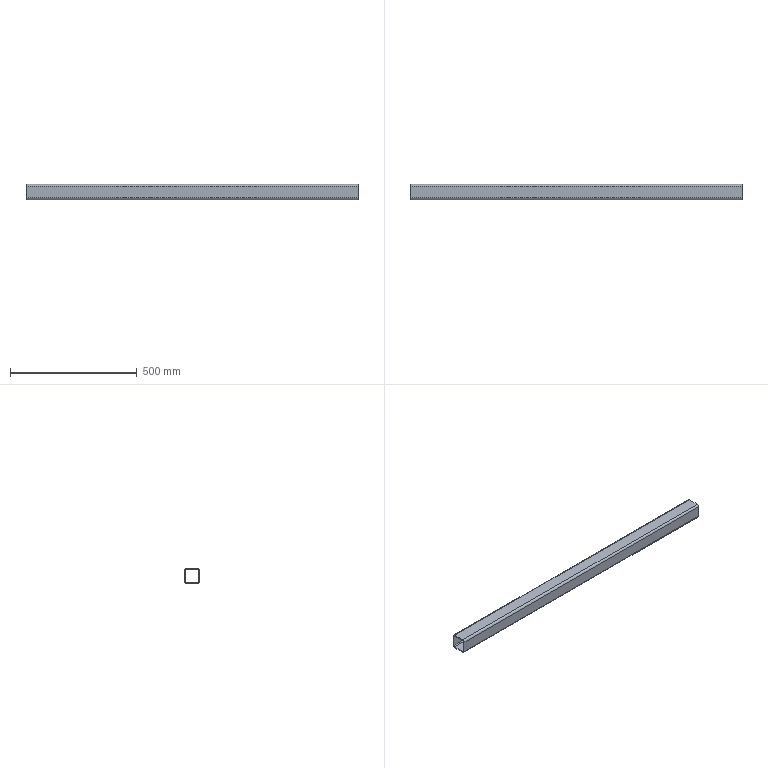Part | SolidWorks | features BaseBody 1 | 1 solid | 18 faces | box 1310 x 60 x 60 mm | volume 1119783 mm3 | plane 10 | cylinder 8 | commonest cylinder face diameters 8 x4 16 x4
STEP:
#1=CARTESIAN_POINT('',(670.,2436.,552.));
#2=VERTEX_POINT('',#1);
#3=CARTESIAN_POINT('',(670.,2436.,508.));
#4=VERTEX_POINT('',#3);
#5=CARTESIAN_POINT('',(670.,2436.,508.));
#6=DIRECTION('',(0.,0.,-1.));
#7=VECTOR('',#6,1000.);
#8=LINE('',#5,#7);
#9=EDGE_CURVE('',#2,#4,#8,.T.);
#10=ORIENTED_EDGE('',*,*,#9,.T.);
#11=CARTESIAN_POINT('',(-640.,2436.,508.));
#12=VERTEX_POINT('',#11);
#13=CARTESIAN_POINT('',(670.,2436.,508.));
#14=DIRECTION('',(-1.,0.,0.));
#15=VECTOR('',#14,1000.);
#16=LINE('',#13,#15);
#17=EDGE_CURVE('',#4,#12,#16,.T.);
#18=ORIENTED_EDGE('',*,*,#17,.T.);
#19=CARTESIAN_POINT('',(-640.,2436.,552.));
#20=VERTEX_POINT('',#19);
#21=CARTESIAN_POINT('',(-640.,2436.,508.));
#22=DIRECTION('',(0.,0.,1.));
#23=VECTOR('',#22,1000.);
#24=LINE('',#21,#23);
#25=EDGE_CURVE('',#12,#20,#24,.T.);
#26=ORIENTED_EDGE('',*,*,#25,.T.);
#27=CARTESIAN_POINT('',(670.,2436.,552.));
#28=DIRECTION('',(1.,0.,0.));
#29=VECTOR('',#28,1000.);
#30=LINE('',#27,#29);
#31=EDGE_CURVE('',#20,#2,#30,.T.);
#32=ORIENTED_EDGE('',*,*,#31,.T.);
#33=EDGE_LOOP('',(#10,#18,#26,#32));
#34=FACE_OUTER_BOUND('',#33,.T.);
#35=CARTESIAN_POINT('',(670.,2436.,508.));
#36=DIRECTION('',(0.,1.,0.));
#37=DIRECTION('',(0.,0.,1.));
#38=AXIS2_PLACEMENT_3D('',#35,#36,#37);
#39=PLANE('',#38);
#40=ADVANCED_FACE('',(#34),#39,.T.);
#41=ORIENTED_EDGE('',*,*,#17,.F.);
#42=CARTESIAN_POINT('',(670.,2440.,504.));
#43=VERTEX_POINT('',#42);
#44=CARTESIAN_POINT('',(670.,2440.,508.));
#45=DIRECTION('',(-1.,0.,0.));
#46=DIRECTION('',(0.,0.,1.));
#47=AXIS2_PLACEMENT_3D('',#44,#45,#46);
#48=CIRCLE('',#47,4.);
#49=EDGE_CURVE('',#43,#4,#48,.T.);
#50=ORIENTED_EDGE('',*,*,#49,.F.);
#51=CARTESIAN_POINT('',(-640.,2440.,504.));
#52=VERTEX_POINT('',#51);
#53=CARTESIAN_POINT('',(670.,2440.,504.));
#54=DIRECTION('',(1.,0.,0.));
#55=VECTOR('',#54,1000.);
#56=LINE('',#53,#55);
#57=EDGE_CURVE('',#52,#43,#56,.T.);
#58=ORIENTED_EDGE('',*,*,#57,.F.);
#59=CARTESIAN_POINT('',(-640.,2440.,508.));
#60=DIRECTION('',(1.,0.,0.));
#61=DIRECTION('',(0.,0.,1.));
#62=AXIS2_PLACEMENT_3D('',#59,#60,#61);
#63=CIRCLE('',#62,4.);
#64=EDGE_CURVE('',#12,#52,#63,.T.);
#65=ORIENTED_EDGE('',*,*,#64,.F.);
#66=EDGE_LOOP('',(#41,#50,#58,#65));
#67=FACE_OUTER_BOUND('',#66,.T.);
#68=CARTESIAN_POINT('',(670.,2440.,508.));
#69=DIRECTION('',(-1.,0.,0.));
#70=DIRECTION('',(0.,0.,1.));
#71=AXIS2_PLACEMENT_3D('',#68,#69,#70);
#72=CYLINDRICAL_SURFACE('',#71,4.);
#73=ADVANCED_FACE('',(#67),#72,.F.);
#74=ORIENTED_EDGE('',*,*,#9,.F.);
#75=CARTESIAN_POINT('',(670.,2440.,556.));
#76=VERTEX_POINT('',#75);
#77=CARTESIAN_POINT('',(670.,2440.,552.));
#78=DIRECTION('',(-1.,0.,0.));
#79=DIRECTION('',(0.,0.,1.));
#80=AXIS2_PLACEMENT_3D('',#77,#78,#79);
#81=CIRCLE('',#80,4.);
#82=EDGE_CURVE('',#2,#76,#81,.T.);
#83=ORIENTED_EDGE('',*,*,#82,.T.);
#84=CARTESIAN_POINT('',(670.,2484.,556.));
#85=VERTEX_POINT('',#84);
#86=CARTESIAN_POINT('',(670.,2484.,556.));
#87=DIRECTION('',(0.,1.,0.));
#88=VECTOR('',#87,1000.);
#89=LINE('',#86,#88);
#90=EDGE_CURVE('',#76,#85,#89,.T.);
#91=ORIENTED_EDGE('',*,*,#90,.T.);
#92=CARTESIAN_POINT('',(670.,2488.,552.));
#93=VERTEX_POINT('',#92);
#94=CARTESIAN_POINT('',(670.,2484.,552.));
#95=DIRECTION('',(-1.,0.,0.));
#96=DIRECTION('',(0.,0.,1.));
#97=AXIS2_PLACEMENT_3D('',#94,#95,#96);
#98=CIRCLE('',#97,4.);
#99=EDGE_CURVE('',#85,#93,#98,.T.);
#100=ORIENTED_EDGE('',*,*,#99,.T.);
#101=CARTESIAN_POINT('',(670.,2488.,508.));
#102=VERTEX_POINT('',#101);
#103=CARTESIAN_POINT('',(670.,2488.,552.));
#104=DIRECTION('',(0.,0.,-1.));
#105=VECTOR('',#104,1000.);
#106=LINE('',#103,#105);
#107=EDGE_CURVE('',#93,#102,#106,.T.);
#108=ORIENTED_EDGE('',*,*,#107,.T.);
#109=CARTESIAN_POINT('',(670.,2484.,504.));
#110=VERTEX_POINT('',#109);
#111=CARTESIAN_POINT('',(670.,2484.,508.));
#112=DIRECTION('',(-1.,0.,0.));
#113=DIRECTION('',(0.,0.,1.));
#114=AXIS2_PLACEMENT_3D('',#111,#112,#113);
#115=CIRCLE('',#114,4.);
#116=EDGE_CURVE('',#102,#110,#115,.T.);
#117=ORIENTED_EDGE('',*,*,#116,.T.);
#118=CARTESIAN_POINT('',(670.,2484.,504.));
#119=DIRECTION('',(0.,-1.,0.));
#120=VECTOR('',#119,1000.);
#121=LINE('',#118,#120);
#122=EDGE_CURVE('',#110,#43,#121,.T.);
#123=ORIENTED_EDGE('',*,*,#122,.T.);
#124=ORIENTED_EDGE('',*,*,#49,.T.);
#125=EDGE_LOOP('',(#74,#83,#91,#100,#108,#117,#123,#124));
#126=FACE_BOUND('',#125,.T.);
#127=CARTESIAN_POINT('',(670.,2492.,508.));
#128=VERTEX_POINT('',#127);
#129=CARTESIAN_POINT('',(670.,2492.,552.));
#130=VERTEX_POINT('',#129);
#131=CARTESIAN_POINT('',(670.,2492.,552.));
#132=DIRECTION('',(0.,0.,1.));
#133=VECTOR('',#132,1000.);
#134=LINE('',#131,#133);
#135=EDGE_CURVE('',#128,#130,#134,.T.);
#136=ORIENTED_EDGE('',*,*,#135,.T.);
#137=CARTESIAN_POINT('',(670.,2484.,560.));
#138=VERTEX_POINT('',#137);
#139=CARTESIAN_POINT('',(670.,2484.,552.));
#140=DIRECTION('',(1.,0.,0.));
#141=DIRECTION('',(0.,0.,1.));
#142=AXIS2_PLACEMENT_3D('',#139,#140,#141);
#143=CIRCLE('',#142,8.);
#144=EDGE_CURVE('',#130,#138,#143,.T.);
#145=ORIENTED_EDGE('',*,*,#144,.T.);
#146=CARTESIAN_POINT('',(670.,2440.,560.));
#147=VERTEX_POINT('',#146);
#148=CARTESIAN_POINT('',(670.,2484.,560.));
#149=DIRECTION('',(0.,-1.,0.));
#150=VECTOR('',#149,1000.);
#151=LINE('',#148,#150);
#152=EDGE_CURVE('',#138,#147,#151,.T.);
#153=ORIENTED_EDGE('',*,*,#152,.T.);
#154=CARTESIAN_POINT('',(670.,2432.,552.));
#155=VERTEX_POINT('',#154);
#156=CARTESIAN_POINT('',(670.,2440.,552.));
#157=DIRECTION('',(1.,0.,0.));
#158=DIRECTION('',(0.,0.,1.));
#159=AXIS2_PLACEMENT_3D('',#156,#157,#158);
#160=CIRCLE('',#159,8.);
#161=EDGE_CURVE('',#147,#155,#160,.T.);
#162=ORIENTED_EDGE('',*,*,#161,.T.);
#163=CARTESIAN_POINT('',(670.,2432.,508.));
#164=VERTEX_POINT('',#163);
#165=CARTESIAN_POINT('',(670.,2432.,552.));
#166=DIRECTION('',(0.,0.,-1.));
#167=VECTOR('',#166,1000.);
#168=LINE('',#165,#167);
#169=EDGE_CURVE('',#155,#164,#168,.T.);
#170=ORIENTED_EDGE('',*,*,#169,.T.);
#171=CARTESIAN_POINT('',(670.,2440.,500.));
#172=VERTEX_POINT('',#171);
#173=CARTESIAN_POINT('',(670.,2440.,508.));
#174=DIRECTION('',(1.,0.,0.));
#175=DIRECTION('',(0.,0.,1.));
#176=AXIS2_PLACEMENT_3D('',#173,#174,#175);
#177=CIRCLE('',#176,8.);
#178=EDGE_CURVE('',#164,#172,#177,.T.);
#179=ORIENTED_EDGE('',*,*,#178,.T.);
#180=CARTESIAN_POINT('',(670.,2484.,500.));
#181=VERTEX_POINT('',#180);
#182=CARTESIAN_POINT('',(670.,2484.,500.));
#183=DIRECTION('',(0.,1.,0.));
#184=VECTOR('',#183,1000.);
#185=LINE('',#182,#184);
#186=EDGE_CURVE('',#172,#181,#185,.T.);
#187=ORIENTED_EDGE('',*,*,#186,.T.);
#188=CARTESIAN_POINT('',(670.,2484.,508.));
#189=DIRECTION('',(1.,0.,0.));
#190=DIRECTION('',(0.,0.,1.));
#191=AXIS2_PLACEMENT_3D('',#188,#189,#190);
#192=CIRCLE('',#191,8.);
#193=EDGE_CURVE('',#181,#128,#192,.T.);
#194=ORIENTED_EDGE('',*,*,#193,.T.);
#195=EDGE_LOOP('',(#136,#145,#153,#162,#170,#179,#187,#194));
#196=FACE_OUTER_BOUND('',#195,.T.);
#197=CARTESIAN_POINT('',(670.,2484.,552.));
#198=DIRECTION('',(1.,0.,0.));
#199=DIRECTION('',(0.,0.,-1.));
#200=AXIS2_PLACEMENT_3D('',#197,#198,#199);
#201=PLANE('',#200);
#202=ADVANCED_FACE('',(#126,#196),#201,.T.);
#203=CARTESIAN_POINT('',(-640.,2440.,556.));
#204=VERTEX_POINT('',#203);
#205=CARTESIAN_POINT('',(670.,2440.,556.));
#206=DIRECTION('',(-1.,0.,0.));
#207=VECTOR('',#206,1000.);
#208=LINE('',#205,#207);
#209=EDGE_CURVE('',#76,#204,#208,.T.);
#210=ORIENTED_EDGE('',*,*,#209,.F.);
#211=ORIENTED_EDGE('',*,*,#82,.F.);
#212=ORIENTED_EDGE('',*,*,#31,.F.);
#213=CARTESIAN_POINT('',(-640.,2440.,552.));
#214=DIRECTION('',(1.,0.,0.));
#215=DIRECTION('',(0.,0.,1.));
#216=AXIS2_PLACEMENT_3D('',#213,#214,#215);
#217=CIRCLE('',#216,4.);
#218=EDGE_CURVE('',#204,#20,#217,.T.);
#219=ORIENTED_EDGE('',*,*,#218,.F.);
#220=EDGE_LOOP('',(#210,#211,#212,#219));
#221=FACE_OUTER_BOUND('',#220,.T.);
#222=CARTESIAN_POINT('',(670.,2440.,552.));
#223=DIRECTION('',(-1.,0.,0.));
#224=DIRECTION('',(0.,0.,1.));
#225=AXIS2_PLACEMENT_3D('',#222,#223,#224);
#226=CYLINDRICAL_SURFACE('',#225,4.);
#227=ADVANCED_FACE('',(#221),#226,.F.);
#228=ORIENTED_EDGE('',*,*,#218,.T.);
#229=ORIENTED_EDGE('',*,*,#25,.F.);
#230=ORIENTED_EDGE('',*,*,#64,.T.);
#231=CARTESIAN_POINT('',(-640.,2484.,504.));
#232=VERTEX_POINT('',#231);
#233=CARTESIAN_POINT('',(-640.,2440.,504.));
#234=DIRECTION('',(0.,1.,0.));
#235=VECTOR('',#234,1000.);
#236=LINE('',#233,#235);
#237=EDGE_CURVE('',#52,#232,#236,.T.);
#238=ORIENTED_EDGE('',*,*,#237,.T.);
#239=CARTESIAN_POINT('',(-640.,2488.,508.));
#240=VERTEX_POINT('',#239);
#241=CARTESIAN_POINT('',(-640.,2484.,508.));
#242=DIRECTION('',(1.,0.,0.));
#243=DIRECTION('',(0.,0.,1.));
#244=AXIS2_PLACEMENT_3D('',#241,#242,#243);
#245=CIRCLE('',#244,4.);
#246=EDGE_CURVE('',#232,#240,#245,.T.);
#247=ORIENTED_EDGE('',*,*,#246,.T.);
#248=CARTESIAN_POINT('',(-640.,2488.,552.));
#249=VERTEX_POINT('',#248);
#250=CARTESIAN_POINT('',(-640.,2488.,-1270.));
#251=DIRECTION('',(0.,0.,1.));
#252=VECTOR('',#251,1000.);
#253=LINE('',#250,#252);
#254=EDGE_CURVE('',#240,#249,#253,.T.);
#255=ORIENTED_EDGE('',*,*,#254,.T.);
#256=CARTESIAN_POINT('',(-640.,2484.,556.));
#257=VERTEX_POINT('',#256);
#258=CARTESIAN_POINT('',(-640.,2484.,552.));
#259=DIRECTION('',(1.,0.,0.));
#260=DIRECTION('',(0.,0.,1.));
#261=AXIS2_PLACEMENT_3D('',#258,#259,#260);
#262=CIRCLE('',#261,4.);
#263=EDGE_CURVE('',#249,#257,#262,.T.);
#264=ORIENTED_EDGE('',*,*,#263,.T.);
#265=CARTESIAN_POINT('',(-640.,2440.,556.));
#266=DIRECTION('',(0.,-1.,0.));
#267=VECTOR('',#266,1000.);
#268=LINE('',#265,#267);
#269=EDGE_CURVE('',#257,#204,#268,.T.);
#270=ORIENTED_EDGE('',*,*,#269,.T.);
#271=EDGE_LOOP('',(#228,#229,#230,#238,#247,#255,#264,#270));
#272=FACE_BOUND('',#271,.T.);
#273=CARTESIAN_POINT('',(-640.,2440.,560.));
#274=VERTEX_POINT('',#273);
#275=CARTESIAN_POINT('',(-640.,2484.,560.));
#276=VERTEX_POINT('',#275);
#277=CARTESIAN_POINT('',(-640.,2440.,560.));
#278=DIRECTION('',(0.,1.,0.));
#279=VECTOR('',#278,1000.);
#280=LINE('',#277,#279);
#281=EDGE_CURVE('',#274,#276,#280,.T.);
#282=ORIENTED_EDGE('',*,*,#281,.T.);
#283=CARTESIAN_POINT('',(-640.,2492.,552.));
#284=VERTEX_POINT('',#283);
#285=CARTESIAN_POINT('',(-640.,2484.,552.));
#286=DIRECTION('',(-1.,0.,0.));
#287=DIRECTION('',(0.,0.,1.));
#288=AXIS2_PLACEMENT_3D('',#285,#286,#287);
#289=CIRCLE('',#288,8.);
#290=EDGE_CURVE('',#276,#284,#289,.T.);
#291=ORIENTED_EDGE('',*,*,#290,.T.);
#292=CARTESIAN_POINT('',(-640.,2492.,508.));
#293=VERTEX_POINT('',#292);
#294=CARTESIAN_POINT('',(-640.,2492.,-1270.));
#295=DIRECTION('',(0.,0.,-1.));
#296=VECTOR('',#295,1000.);
#297=LINE('',#294,#296);
#298=EDGE_CURVE('',#284,#293,#297,.T.);
#299=ORIENTED_EDGE('',*,*,#298,.T.);
#300=CARTESIAN_POINT('',(-640.,2484.,500.));
#301=VERTEX_POINT('',#300);
#302=CARTESIAN_POINT('',(-640.,2484.,508.));
#303=DIRECTION('',(-1.,0.,0.));
#304=DIRECTION('',(0.,0.,1.));
#305=AXIS2_PLACEMENT_3D('',#302,#303,#304);
#306=CIRCLE('',#305,8.);
#307=EDGE_CURVE('',#293,#301,#306,.T.);
#308=ORIENTED_EDGE('',*,*,#307,.T.);
#309=CARTESIAN_POINT('',(-640.,2440.,500.));
#310=VERTEX_POINT('',#309);
#311=CARTESIAN_POINT('',(-640.,2440.,500.));
#312=DIRECTION('',(0.,-1.,0.));
#313=VECTOR('',#312,1000.);
#314=LINE('',#311,#313);
#315=EDGE_CURVE('',#301,#310,#314,.T.);
#316=ORIENTED_EDGE('',*,*,#315,.T.);
#317=CARTESIAN_POINT('',(-640.,2432.,508.));
#318=VERTEX_POINT('',#317);
#319=CARTESIAN_POINT('',(-640.,2440.,508.));
#320=DIRECTION('',(-1.,0.,0.));
#321=DIRECTION('',(0.,0.,1.));
#322=AXIS2_PLACEMENT_3D('',#319,#320,#321);
#323=CIRCLE('',#322,8.);
#324=EDGE_CURVE('',#310,#318,#323,.T.);
#325=ORIENTED_EDGE('',*,*,#324,.T.);
#326=CARTESIAN_POINT('',(-640.,2432.,552.));
#327=VERTEX_POINT('',#326);
#328=CARTESIAN_POINT('',(-640.,2432.,-1270.));
#329=DIRECTION('',(0.,0.,1.));
#330=VECTOR('',#329,1000.);
#331=LINE('',#328,#330);
#332=EDGE_CURVE('',#318,#327,#331,.T.);
#333=ORIENTED_EDGE('',*,*,#332,.T.);
#334=CARTESIAN_POINT('',(-640.,2440.,552.));
#335=DIRECTION('',(-1.,0.,0.));
#336=DIRECTION('',(0.,0.,1.));
#337=AXIS2_PLACEMENT_3D('',#334,#335,#336);
#338=CIRCLE('',#337,8.);
#339=EDGE_CURVE('',#327,#274,#338,.T.);
#340=ORIENTED_EDGE('',*,*,#339,.T.);
#341=EDGE_LOOP('',(#282,#291,#299,#308,#316,#325,#333,#340));
#342=FACE_OUTER_BOUND('',#341,.T.);
#343=CARTESIAN_POINT('',(-640.,2440.,-1270.));
#344=DIRECTION('',(-1.,0.,0.));
#345=DIRECTION('',(0.,0.,1.));
#346=AXIS2_PLACEMENT_3D('',#343,#344,#345);
#347=PLANE('',#346);
#348=ADVANCED_FACE('',(#272,#342),#347,.T.);
#349=ORIENTED_EDGE('',*,*,#122,.F.);
#350=CARTESIAN_POINT('',(670.,2484.,504.));
#351=DIRECTION('',(-1.,0.,0.));
#352=VECTOR('',#351,1000.);
#353=LINE('',#350,#352);
#354=EDGE_CURVE('',#110,#232,#353,.T.);
#355=ORIENTED_EDGE('',*,*,#354,.T.);
#356=ORIENTED_EDGE('',*,*,#237,.F.);
#357=ORIENTED_EDGE('',*,*,#57,.T.);
#358=EDGE_LOOP('',(#349,#355,#356,#357));
#359=FACE_OUTER_BOUND('',#358,.T.);
#360=CARTESIAN_POINT('',(670.,2440.,504.));
#361=DIRECTION('',(0.,0.,1.));
#362=DIRECTION('',(1.,0.,0.));
#363=AXIS2_PLACEMENT_3D('',#360,#361,#362);
#364=PLANE('',#363);
#365=ADVANCED_FACE('',(#359),#364,.T.);
#366=ORIENTED_EDGE('',*,*,#354,.F.);
#367=ORIENTED_EDGE('',*,*,#116,.F.);
#368=CARTESIAN_POINT('',(670.,2488.,508.));
#369=DIRECTION('',(1.,0.,0.));
#370=VECTOR('',#369,1000.);
#371=LINE('',#368,#370);
#372=EDGE_CURVE('',#240,#102,#371,.T.);
#373=ORIENTED_EDGE('',*,*,#372,.F.);
#374=ORIENTED_EDGE('',*,*,#246,.F.);
#375=EDGE_LOOP('',(#366,#367,#373,#374));
#376=FACE_OUTER_BOUND('',#375,.T.);
#377=CARTESIAN_POINT('',(670.,2484.,508.));
#378=DIRECTION('',(-1.,0.,0.));
#379=DIRECTION('',(0.,0.,1.));
#380=AXIS2_PLACEMENT_3D('',#377,#378,#379);
#381=CYLINDRICAL_SURFACE('',#380,4.);
#382=ADVANCED_FACE('',(#376),#381,.F.);
#383=ORIENTED_EDGE('',*,*,#107,.F.);
#384=CARTESIAN_POINT('',(670.,2488.,552.));
#385=DIRECTION('',(-1.,0.,0.));
#386=VECTOR('',#385,1000.);
#387=LINE('',#384,#386);
#388=EDGE_CURVE('',#93,#249,#387,.T.);
#389=ORIENTED_EDGE('',*,*,#388,.T.);
#390=ORIENTED_EDGE('',*,*,#254,.F.);
#391=ORIENTED_EDGE('',*,*,#372,.T.);
#392=EDGE_LOOP('',(#383,#389,#390,#391));
#393=FACE_OUTER_BOUND('',#392,.T.);
#394=CARTESIAN_POINT('',(670.,2488.,552.));
#395=DIRECTION('',(0.,-1.,0.));
#396=DIRECTION('',(0.,0.,-1.));
#397=AXIS2_PLACEMENT_3D('',#394,#395,#396);
#398=PLANE('',#397);
#399=ADVANCED_FACE('',(#393),#398,.T.);
#400=ORIENTED_EDGE('',*,*,#388,.F.);
#401=ORIENTED_EDGE('',*,*,#99,.F.);
#402=CARTESIAN_POINT('',(670.,2484.,556.));
#403=DIRECTION('',(1.,0.,0.));
#404=VECTOR('',#403,1000.);
#405=LINE('',#402,#404);
#406=EDGE_CURVE('',#257,#85,#405,.T.);
#407=ORIENTED_EDGE('',*,*,#406,.F.);
#408=ORIENTED_EDGE('',*,*,#263,.F.);
#409=EDGE_LOOP('',(#400,#401,#407,#408));
#410=FACE_OUTER_BOUND('',#409,.T.);
#411=CARTESIAN_POINT('',(670.,2484.,552.));
#412=DIRECTION('',(-1.,0.,0.));
#413=DIRECTION('',(0.,0.,1.));
#414=AXIS2_PLACEMENT_3D('',#411,#412,#413);
#415=CYLINDRICAL_SURFACE('',#414,4.);
#416=ADVANCED_FACE('',(#410),#415,.F.);
#417=ORIENTED_EDGE('',*,*,#90,.F.);
#418=ORIENTED_EDGE('',*,*,#209,.T.);
#419=ORIENTED_EDGE('',*,*,#269,.F.);
#420=ORIENTED_EDGE('',*,*,#406,.T.);
#421=EDGE_LOOP('',(#417,#418,#419,#420));
#422=FACE_OUTER_BOUND('',#421,.T.);
#423=CARTESIAN_POINT('',(670.,2484.,556.));
#424=DIRECTION('',(0.,0.,-1.));
#425=DIRECTION('',(-1.,0.,0.));
#426=AXIS2_PLACEMENT_3D('',#423,#424,#425);
#427=PLANE('',#426);
#428=ADVANCED_FACE('',(#422),#427,.T.);
#429=CARTESIAN_POINT('',(670.,2492.,552.));
#430=DIRECTION('',(-1.,0.,0.));
#431=VECTOR('',#430,1000.);
#432=LINE('',#429,#431);
#433=EDGE_CURVE('',#130,#284,#432,.T.);
#434=ORIENTED_EDGE('',*,*,#433,.T.);
#435=ORIENTED_EDGE('',*,*,#290,.F.);
#436=CARTESIAN_POINT('',(670.,2484.,560.));
#437=DIRECTION('',(1.,0.,0.));
#438=VECTOR('',#437,1000.);
#439=LINE('',#436,#438);
#440=EDGE_CURVE('',#276,#138,#439,.T.);
#441=ORIENTED_EDGE('',*,*,#440,.T.);
#442=ORIENTED_EDGE('',*,*,#144,.F.);
#443=EDGE_LOOP('',(#434,#435,#441,#442));
#444=FACE_OUTER_BOUND('',#443,.T.);
#445=CARTESIAN_POINT('',(670.,2484.,552.));
#446=DIRECTION('',(-1.,0.,0.));
#447=DIRECTION('',(0.,0.,1.));
#448=AXIS2_PLACEMENT_3D('',#445,#446,#447);
#449=CYLINDRICAL_SURFACE('',#448,8.);
#450=ADVANCED_FACE('',(#444),#449,.T.);
#451=ORIENTED_EDGE('',*,*,#135,.F.);
#452=CARTESIAN_POINT('',(670.,2492.,508.));
#453=DIRECTION('',(1.,0.,0.));
#454=VECTOR('',#453,1000.);
#455=LINE('',#452,#454);
#456=EDGE_CURVE('',#293,#128,#455,.T.);
#457=ORIENTED_EDGE('',*,*,#456,.F.);
#458=ORIENTED_EDGE('',*,*,#298,.F.);
#459=ORIENTED_EDGE('',*,*,#433,.F.);
#460=EDGE_LOOP('',(#451,#457,#458,#459));
#461=FACE_OUTER_BOUND('',#460,.T.);
#462=CARTESIAN_POINT('',(670.,2492.,552.));
#463=DIRECTION('',(0.,-1.,0.));
#464=DIRECTION('',(0.,0.,-1.));
#465=AXIS2_PLACEMENT_3D('',#462,#463,#464);
#466=PLANE('',#465);
#467=ADVANCED_FACE('',(#461),#466,.F.);
#468=CARTESIAN_POINT('',(670.,2484.,500.));
#469=DIRECTION('',(-1.,0.,0.));
#470=VECTOR('',#469,1000.);
#471=LINE('',#468,#470);
#472=EDGE_CURVE('',#181,#301,#471,.T.);
#473=ORIENTED_EDGE('',*,*,#472,.T.);
#474=ORIENTED_EDGE('',*,*,#307,.F.);
#475=ORIENTED_EDGE('',*,*,#456,.T.);
#476=ORIENTED_EDGE('',*,*,#193,.F.);
#477=EDGE_LOOP('',(#473,#474,#475,#476));
#478=FACE_OUTER_BOUND('',#477,.T.);
#479=CARTESIAN_POINT('',(670.,2484.,508.));
#480=DIRECTION('',(-1.,0.,0.));
#481=DIRECTION('',(0.,0.,1.));
#482=AXIS2_PLACEMENT_3D('',#479,#480,#481);
#483=CYLINDRICAL_SURFACE('',#482,8.);
#484=ADVANCED_FACE('',(#478),#483,.T.);
#485=ORIENTED_EDGE('',*,*,#186,.F.);
#486=CARTESIAN_POINT('',(670.,2440.,500.));
#487=DIRECTION('',(1.,0.,0.));
#488=VECTOR('',#487,1000.);
#489=LINE('',#486,#488);
#490=EDGE_CURVE('',#310,#172,#489,.T.);
#491=ORIENTED_EDGE('',*,*,#490,.F.);
#492=ORIENTED_EDGE('',*,*,#315,.F.);
#493=ORIENTED_EDGE('',*,*,#472,.F.);
#494=EDGE_LOOP('',(#485,#491,#492,#493));
#495=FACE_OUTER_BOUND('',#494,.T.);
#496=CARTESIAN_POINT('',(670.,2440.,500.));
#497=DIRECTION('',(0.,0.,1.));
#498=DIRECTION('',(1.,0.,0.));
#499=AXIS2_PLACEMENT_3D('',#496,#497,#498);
#500=PLANE('',#499);
#501=ADVANCED_FACE('',(#495),#500,.F.);
#502=CARTESIAN_POINT('',(670.,2432.,508.));
#503=DIRECTION('',(-1.,0.,0.));
#504=VECTOR('',#503,1000.);
#505=LINE('',#502,#504);
#506=EDGE_CURVE('',#164,#318,#505,.T.);
#507=ORIENTED_EDGE('',*,*,#506,.T.);
#508=ORIENTED_EDGE('',*,*,#324,.F.);
#509=ORIENTED_EDGE('',*,*,#490,.T.);
#510=ORIENTED_EDGE('',*,*,#178,.F.);
#511=EDGE_LOOP('',(#507,#508,#509,#510));
#512=FACE_OUTER_BOUND('',#511,.T.);
#513=CARTESIAN_POINT('',(670.,2440.,508.));
#514=DIRECTION('',(-1.,0.,0.));
#515=DIRECTION('',(0.,0.,1.));
#516=AXIS2_PLACEMENT_3D('',#513,#514,#515);
#517=CYLINDRICAL_SURFACE('',#516,8.);
#518=ADVANCED_FACE('',(#512),#517,.T.);
#519=ORIENTED_EDGE('',*,*,#169,.F.);
#520=CARTESIAN_POINT('',(670.,2432.,552.));
#521=DIRECTION('',(1.,0.,0.));
#522=VECTOR('',#521,1000.);
#523=LINE('',#520,#522);
#524=EDGE_CURVE('',#327,#155,#523,.T.);
#525=ORIENTED_EDGE('',*,*,#524,.F.);
#526=ORIENTED_EDGE('',*,*,#332,.F.);
#527=ORIENTED_EDGE('',*,*,#506,.F.);
#528=EDGE_LOOP('',(#519,#525,#526,#527));
#529=FACE_OUTER_BOUND('',#528,.T.);
#530=CARTESIAN_POINT('',(670.,2432.,508.));
#531=DIRECTION('',(0.,1.,0.));
#532=DIRECTION('',(0.,0.,1.));
#533=AXIS2_PLACEMENT_3D('',#530,#531,#532);
#534=PLANE('',#533);
#535=ADVANCED_FACE('',(#529),#534,.F.);
#536=CARTESIAN_POINT('',(670.,2440.,560.));
#537=DIRECTION('',(-1.,0.,0.));
#538=VECTOR('',#537,1000.);
#539=LINE('',#536,#538);
#540=EDGE_CURVE('',#147,#274,#539,.T.);
#541=ORIENTED_EDGE('',*,*,#540,.T.);
#542=ORIENTED_EDGE('',*,*,#339,.F.);
#543=ORIENTED_EDGE('',*,*,#524,.T.);
#544=ORIENTED_EDGE('',*,*,#161,.F.);
#545=EDGE_LOOP('',(#541,#542,#543,#544));
#546=FACE_OUTER_BOUND('',#545,.T.);
#547=CARTESIAN_POINT('',(670.,2440.,552.));
#548=DIRECTION('',(-1.,0.,0.));
#549=DIRECTION('',(0.,0.,1.));
#550=AXIS2_PLACEMENT_3D('',#547,#548,#549);
#551=CYLINDRICAL_SURFACE('',#550,8.);
#552=ADVANCED_FACE('',(#546),#551,.T.);
#553=ORIENTED_EDGE('',*,*,#152,.F.);
#554=ORIENTED_EDGE('',*,*,#440,.F.);
#555=ORIENTED_EDGE('',*,*,#281,.F.);
#556=ORIENTED_EDGE('',*,*,#540,.F.);
#557=EDGE_LOOP('',(#553,#554,#555,#556));
#558=FACE_OUTER_BOUND('',#557,.T.);
#559=CARTESIAN_POINT('',(670.,2484.,560.));
#560=DIRECTION('',(0.,0.,-1.));
#561=DIRECTION('',(-1.,0.,0.));
#562=AXIS2_PLACEMENT_3D('',#559,#560,#561);
#563=PLANE('',#562);
#564=ADVANCED_FACE('',(#558),#563,.F.);
#565=CLOSED_SHELL('',(#40,#73,#202,#227,#348,#365,#382,#399,#416,#428,#450,#467,#484,#501,#518,#535,#552,#564));
#566=MANIFOLD_SOLID_BREP('',#565);
#567=CARTESIAN_POINT('',(0.,0.,0.));
#568=DIRECTION('',(0.,0.,1.));
#569=DIRECTION('',(1.,0.,0.));
#570=AXIS2_PLACEMENT_3D('',#567,#568,#569);
#571=(LENGTH_UNIT()NAMED_UNIT(*)SI_UNIT(.MILLI.,.METRE.));
#572=UNCERTAINTY_MEASURE_WITH_UNIT(LENGTH_MEASURE(0.00001),#571,'','');
#573=(NAMED_UNIT(*)PLANE_ANGLE_UNIT()SI_UNIT($,.RADIAN.));
#574=(NAMED_UNIT(*)SI_UNIT($,.STERADIAN.)SOLID_ANGLE_UNIT());
#575=(GEOMETRIC_REPRESENTATION_CONTEXT(3)GLOBAL_UNCERTAINTY_ASSIGNED_CONTEXT((#572))GLOBAL_UNIT_ASSIGNED_CONTEXT((#571,#573,#574))REPRESENTATION_CONTEXT('',''));
#576=ADVANCED_BREP_SHAPE_REPRESENTATION('',(#566,#570),#575);